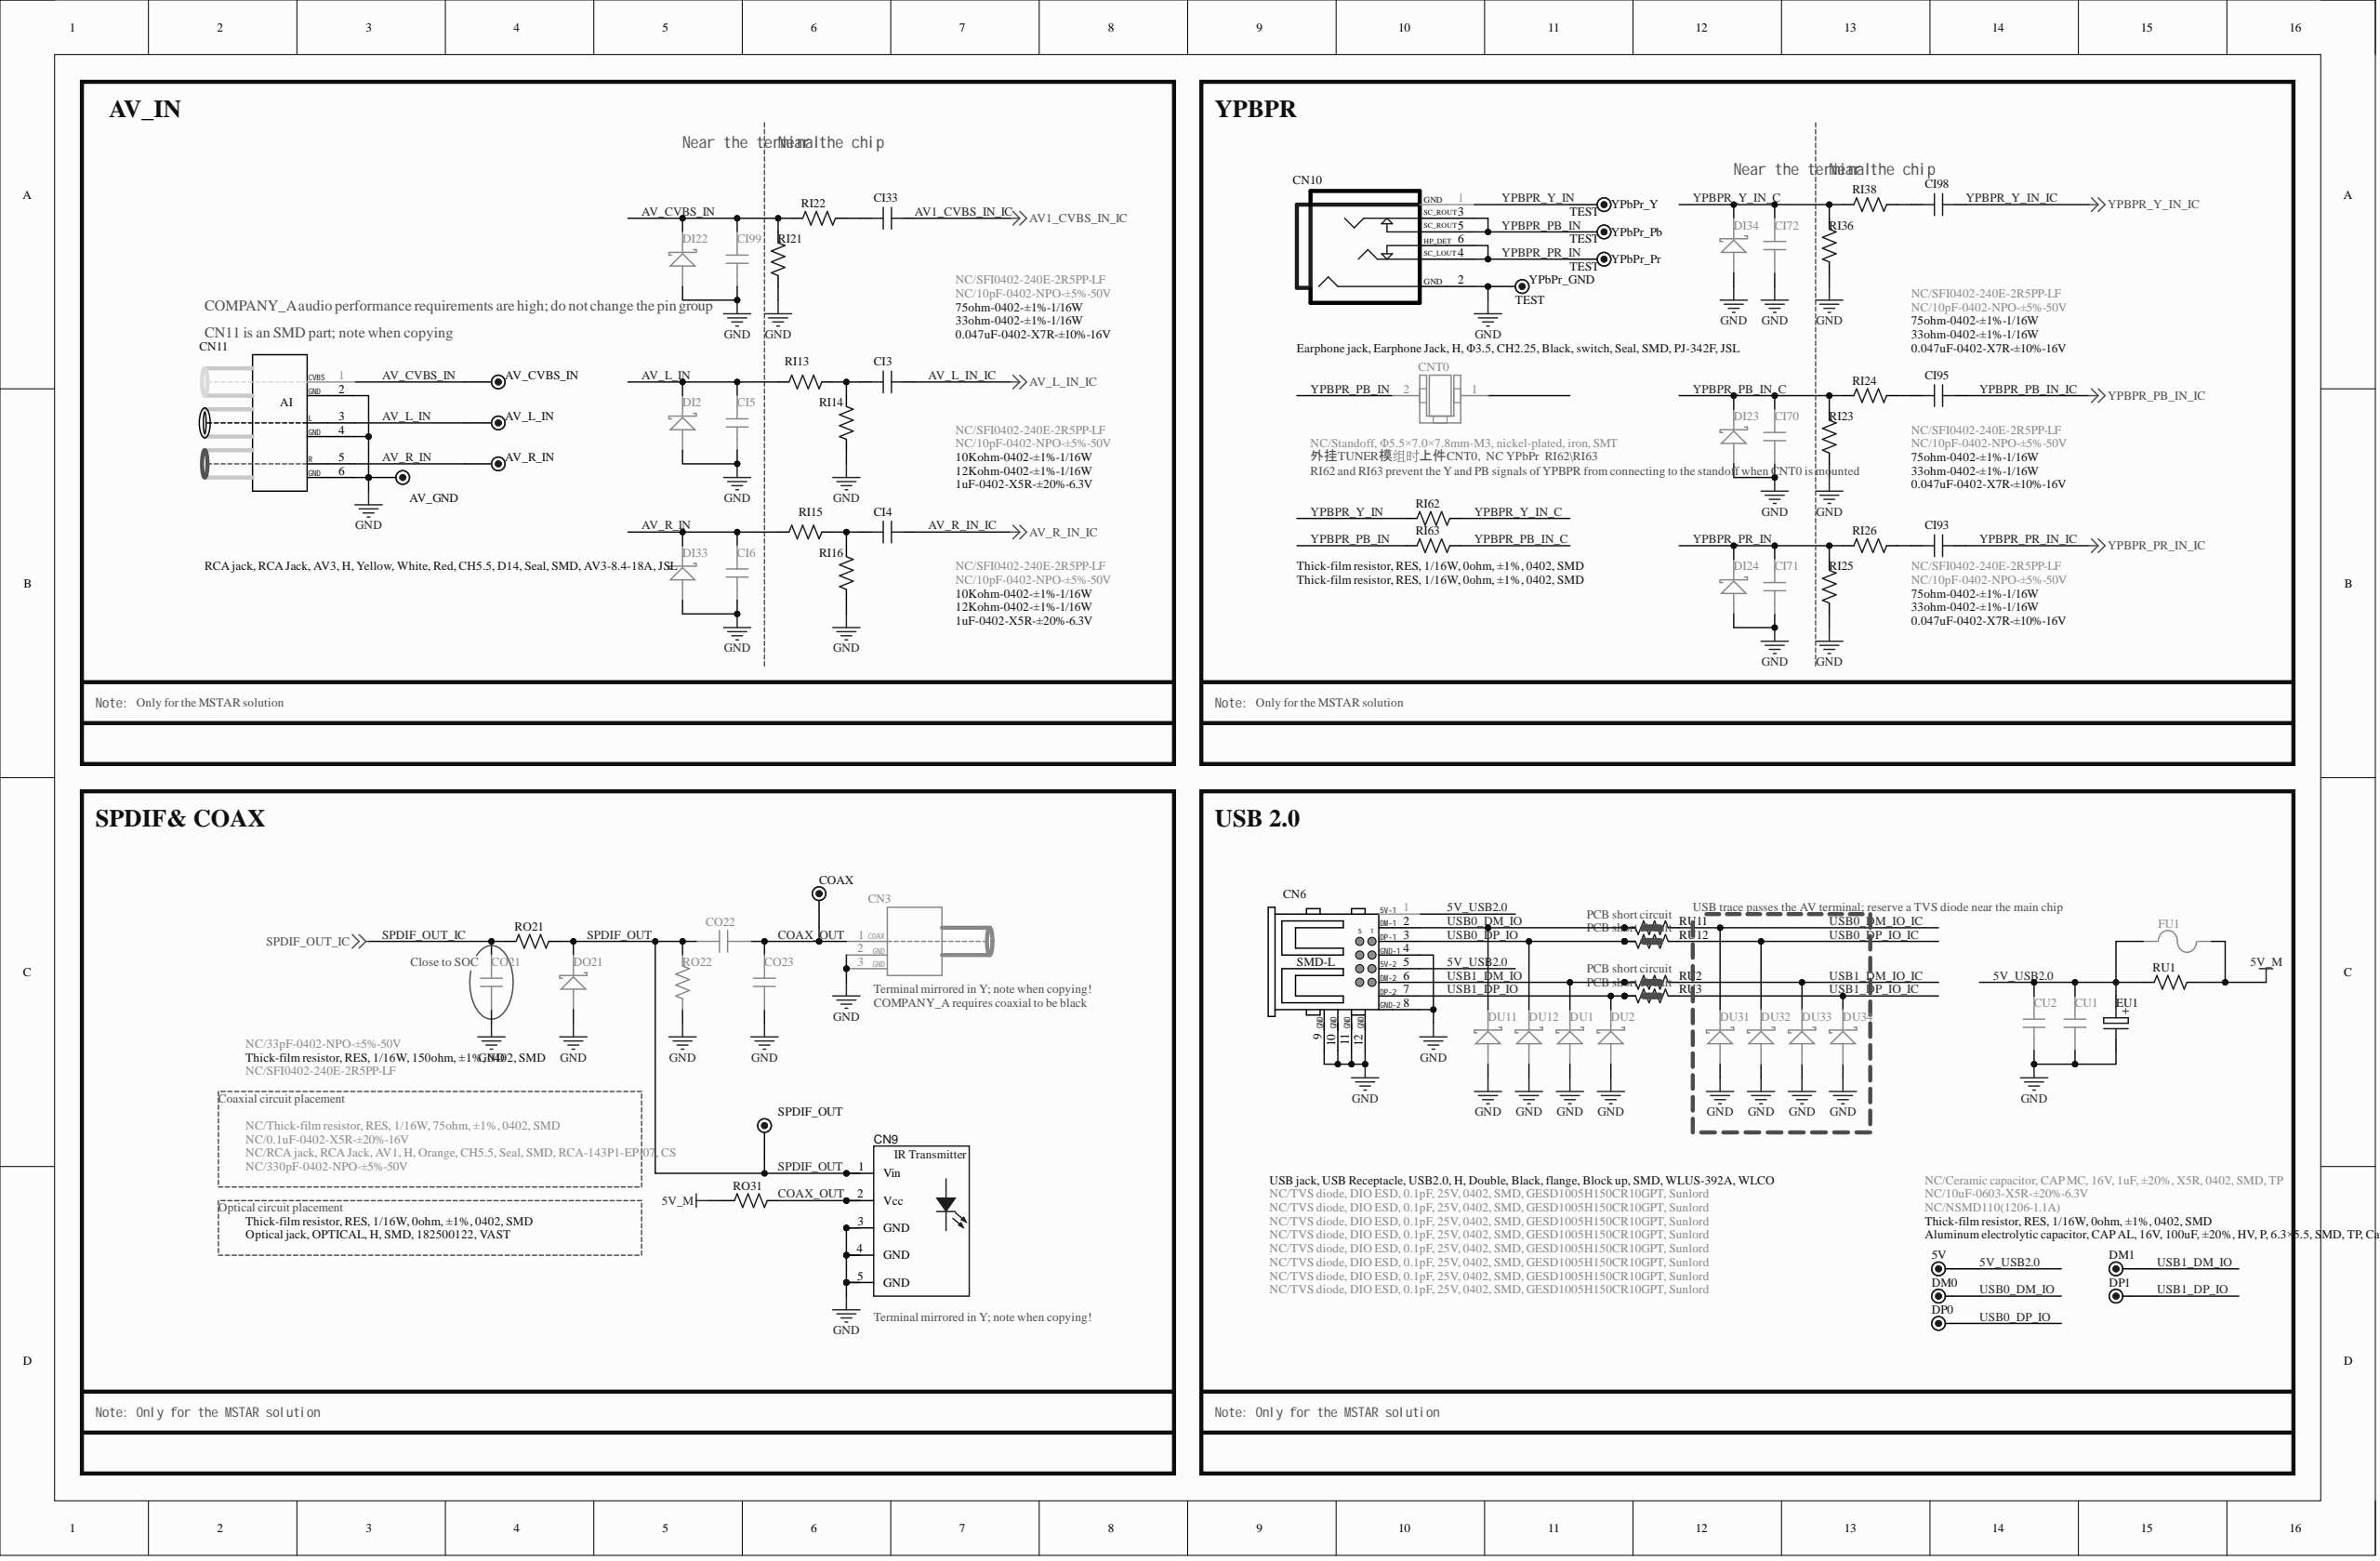Circuit board | Altium Designer | 541 parts | 263 nets | one sheet of the schematic
Parts on this sheet (reference | value | footprint):
5V | DM0 | TP
AV_CVBS_IN | TEST | TP
AV_GND | TEST | TP
AV_L_IN | TEST | TP
AV_R_IN | TEST | TP
CI3 | 1uF-0402-X5R-±20%-6.3V | C0402
CI4 | 1uF-0402-X5R-±20%-6.3V | C0402
CI5 | NC/10pF-0402-NPO-±5%-50V | C0402
CI6 | NC/10pF-0402-NPO-±5%-50V | C0402
CI33 | 0.047uF-0402-X7R-±10%-16V | C0402
CI70 | NC/10pF-0402-NPO-±5%-50V | C0402
CI71 | NC/10pF-0402-NPO-±5%-50V | C0402
CI72 | NC/10pF-0402-NPO-±5%-50V | C0402
CI93 | 0.047uF-0402-X7R-±10%-16V | C0402
CI95 | 0.047uF-0402-X7R-±10%-16V | C0402
CI98 | 0.047uF-0402-X7R-±10%-16V | C0402
CI99 | NC/10pF-0402-NPO-±5%-50V | C0402
CN3 | NC/RCA jack, RCA Jack, AV1, H, Orange, CH5.5, Seal, SMD, RCA-143P1-EP-07, CS | AV1-H-4-S
CN6 | USB jack, USB Receptacle, USB2.0, H, Double, Black, flange, Block up, SMD, WLUS-392A, WLCO | USB2-HS-1
CN9 | Optical jack, OPTICAL, H, SMD, 182500122, VAST | OPTICAL-HS-1
CN10 | Earphone jack, Earphone Jack, H, F3.5, CH2.25, Black, switch, Seal, SMD, PJ-342F, JSL | PHONE-HS-29
CN11 | RCA jack, RCA Jack, AV3, H, Yellow, White, Red, CH5.5, D14, Seal, SMD, AV3-8.4-18A, JSL | AV3-H14-15-S
CNT0 | NC/Standoff, F5.5×7.0×7.8mm-M3, nickel-plated, iron, SMT | FIX-5.5*7.0*7.8-S-1
CO21 | NC/33pF-0402-NPO-±5%-50V | C0402
CO22 | NC/0.1uF-0402-X5R-±20%-16V | C0402
CO23 | NC/330pF-0402-NPO-±5%-50V | C0402
COAX | TEST | TP
CU1 | NC/10uF-0603-X5R-±20%-6.3V | C0603
CU2 | NC/Ceramic capacitor, CAP MC, 16V, 1uF, ±20%, X5R, 0402, SMD, TP | C0402
DI2 | NC/SFI0402-240E-2R5PP-LF | DIODE-S0402
DI22 | NC/SFI0402-240E-2R5PP-LF | DIODE-S0402
DI23 | NC/SFI0402-240E-2R5PP-LF | DIODE-S0402
DI24 | NC/SFI0402-240E-2R5PP-LF | DIODE-S0402
DI33 | NC/SFI0402-240E-2R5PP-LF | DIODE-S0402
DI34 | NC/SFI0402-240E-2R5PP-LF | DIODE-S0402
DM0 | DM0 | TP
DM1 | DM0 | TP
DO21 | NC/SFI0402-240E-2R5PP-LF | DIODE-S0402
DP0 | DM0 | TP
DP1 | DM0 | TP
DU1 | NC/TVS diode, DIO ESD, 0.1pF, 25V, 0402, SMD, GESD1005H150CR10GPT, Sunlord | DIODE-S0402
DU2 | NC/TVS diode, DIO ESD, 0.1pF, 25V, 0402, SMD, GESD1005H150CR10GPT, Sunlord | DIODE-S0402
DU11 | NC/TVS diode, DIO ESD, 0.1pF, 25V, 0402, SMD, GESD1005H150CR10GPT, Sunlord | DIODE-S0402
DU12 | NC/TVS diode, DIO ESD, 0.1pF, 25V, 0402, SMD, GESD1005H150CR10GPT, Sunlord | DIODE-S0402
DU31 | NC/TVS diode, DIO ESD, 0.1pF, 25V, 0402, SMD, GESD1005H150CR10GPT, Sunlord | DIODE-S0402
DU32 | NC/TVS diode, DIO ESD, 0.1pF, 25V, 0402, SMD, GESD1005H150CR10GPT, Sunlord | DIODE-S0402
DU33 | NC/TVS diode, DIO ESD, 0.1pF, 25V, 0402, SMD, GESD1005H150CR10GPT, Sunlord | DIODE-S0402
DU34 | NC/TVS diode, DIO ESD, 0.1pF, 25V, 0402, SMD, GESD1005H150CR10GPT, Sunlord | DIODE-S0402
FU1 | NC/NSMD110(1206-1.1A) | FUSE1.1A-S
IR | DM0 | TP
RI13 | 10Kohm-0402-±1%-1/16W | R0402
RI14 | 12Kohm-0402-±1%-1/16W | R0402
RI15 | 10Kohm-0402-±1%-1/16W | R0402
RI16 | 12Kohm-0402-±1%-1/16W | R0402
RI21 | 75ohm-0402-±1%-1/16W | R0402
RI22 | 33ohm-0402-±1%-1/16W | R0402
RI23 | 75ohm-0402-±1%-1/16W | R0402
RI24 | 33ohm-0402-±1%-1/16W | R0402
RI25 | 75ohm-0402-±1%-1/16W | R0402
RI26 | 33ohm-0402-±1%-1/16W | R0402
RI36 | 75ohm-0402-±1%-1/16W | R0402
RI38 | 33ohm-0402-±1%-1/16W | R0402
RI62 | Thick-film resistor, RES, 1/16W, 0ohm, ±1%, 0402, SMD | R0402
RI63 | Thick-film resistor, RES, 1/16W, 0ohm, ±1%, 0402, SMD | R0402
RO21 | Thick-film resistor, RES, 1/16W, 150ohm, ±1%, 0402, SMD | R0402
RO22 | NC/Thick-film resistor, RES, 1/16W, 75ohm, ±1%, 0402, SMD | R0402
RO31 | Thick-film resistor, RES, 1/16W, 0ohm, ±1%, 0402, SMD | R0402
RU1 | Thick-film resistor, RES, 1/16W, 0ohm, ±1%, 0402, SMD | R0402
RU2 | NC/0ohm-0402-PCB | R0402SC
RU3 | NC/0ohm-0402-PCB | R0402SC
RU11 | NC/0ohm-0402-PCB | R0402SC
RU12 | NC/0ohm-0402-PCB | R0402SC
SPDIF_OUT | TEST | TP
YPbPr_GND | TEST | TP
YPbPr_Pb | TEST | TP
YPbPr_Pr | TEST | TP
YPbPr_Y | TEST | TP
Nets of these parts (net: part-pin ...):
YPBPR_Y_IN_IC: CI98-2
YPBPR_Y_IN_C: CI72-2 DI34-K RI36-2 RI38-1 RI62-1
YPBPR_Y_IN: CN10-1 RI62-2 YPbPr_Y-1
YPBPR_PR_IN_IC: CI93-2
YPBPR_PR_IN: CI71-2 CN10-4 CN10-6 DI24-K RI25-2 RI26-1 YPbPr_Pr-1
YPBPR_PB_IN_IC: CI95-2
YPBPR_PB_IN_C: CI70-2 DI23-K RI23-2 RI24-1 RI63-1
YPBPR_PB_IN: CN10-3 CN10-5 CNT0-2 RI63-2 YPbPr_Pb-1
USB1_DP_IO_IC: DU34-K RU3-1
USB1_DP_IO: CN6-7 DP1-1 DU2-K RU3-2 RU3-3
USB1_DM_IO_IC: DU33-K RU2-1
USB1_DM_IO: CN6-6 DM1-1 DU1-K RU2-2 RU2-3
USB0_DP_IO_IC: DU32-K RU12-1
USB0_DP_IO: CN6-3 DP0-1 DU12-K RU12-2 RU12-3
USB0_DM_IO_IC: DU31-K RU11-1
USB0_DM_IO: CN6-2 DM0-1 DU11-K RU11-2 RU11-3
SPDIF_OUT_IC: CO21-2 RO21-1
SPDIF_OUT: CN9-1 CO22-1 DO21-K RO21-2 RO22-2 SPDIF_OUT-1
NetCI98_1: CI98-1 RI38-2
NetCI95_1: CI95-1 RI24-2
NetCI93_1: CI93-1 RI26-2
NetCI33_1: CI33-1 RI22-2
NetCI4_2: CI4-2 RI15-1 RI16-1
NetCI3_2: CI3-2 RI13-1 RI14-1
IR: IR-1
GND: AV_GND-1 CI5-1 CI6-1 CI70-1 CI71-1 CI72-1 CI99-1 CN3-2 CN3-3 CN6-4 CN6-8 CN6-9 CN6-10 CN6-11 CN6-12 CN9-3 CN9-4 CN9-5 CN10-2 CN11-2 CN11-4 CN11-6 CO21-1 CO23-1 CU1-1 CU2-2 DI2-A DI22-A DI23-A DI24-A DI33-A DI34-A DO21-A DU1-A DU2-A DU11-A DU12-A DU31-A DU32-A DU33-A DU34-A RI14-2 RI16-2 RI21-1 RI23-1 RI25-1 RI36-1 RO22-1 YPbPr_GND-1
COAX_OUT: CN3-1 CN9-2 CO22-2 CO23-2 COAX-1 RO31-1
AV_R_IN_IC: CI4-1
AV_R_IN: AV_R_IN-1 CI6-2 CN11-5 DI33-K RI15-2
AV_L_IN_IC: CI3-1
AV_L_IN: AV_L_IN-1 CI5-2 CN11-3 DI2-K RI13-2
AV_CVBS_IN: AV_CVBS_IN-1 CI99-2 CN11-1 DI22-K RI21-2 RI22-1
AV1_CVBS_IN_IC: CI33-2
5V_USB2.0: 5V-1 CN6-1 CN6-5 CU1-2 CU2-1 FU1-1 RU1-1
5V_M: FU1-2 RO31-2 RU1-2